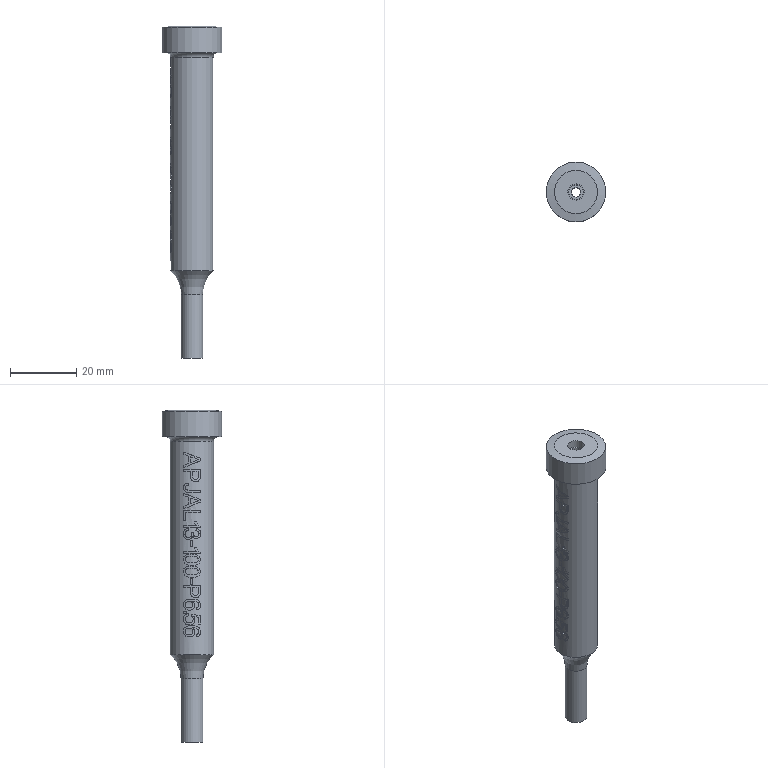Part | STEP file | APJAL13-100-P6.56_2_id106_x_t | 1 solid | 213 faces | box 18 x 18 x 100 mm | volume 10594 mm3 | plane 122 | cylinder 88 | torus 2 | cone 1 | commonest cylinder face diameters 12.8 x17 13 x9 1.745 x2 1.803 x2 1.952 x2 2.008 x2